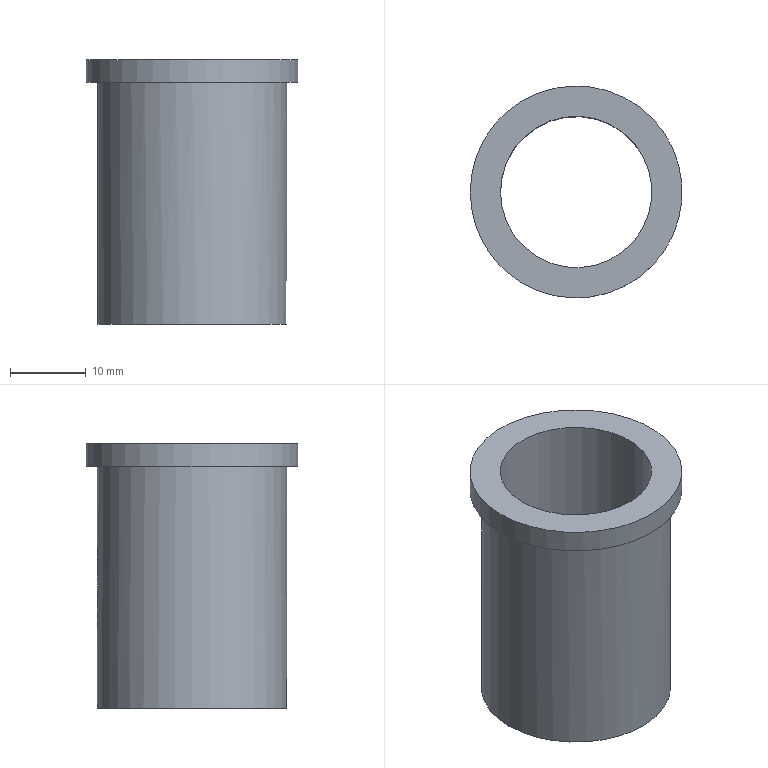Part | STEP file | SGBH 20-16_id490_x_t | 1 solid | 144 faces | box 28 x 28 x 35 mm | volume 6555 mm3 | other 84 | plane 54 | cylinder 6 | commonest cylinder face diameters 25 x4 20 x1 28 x1